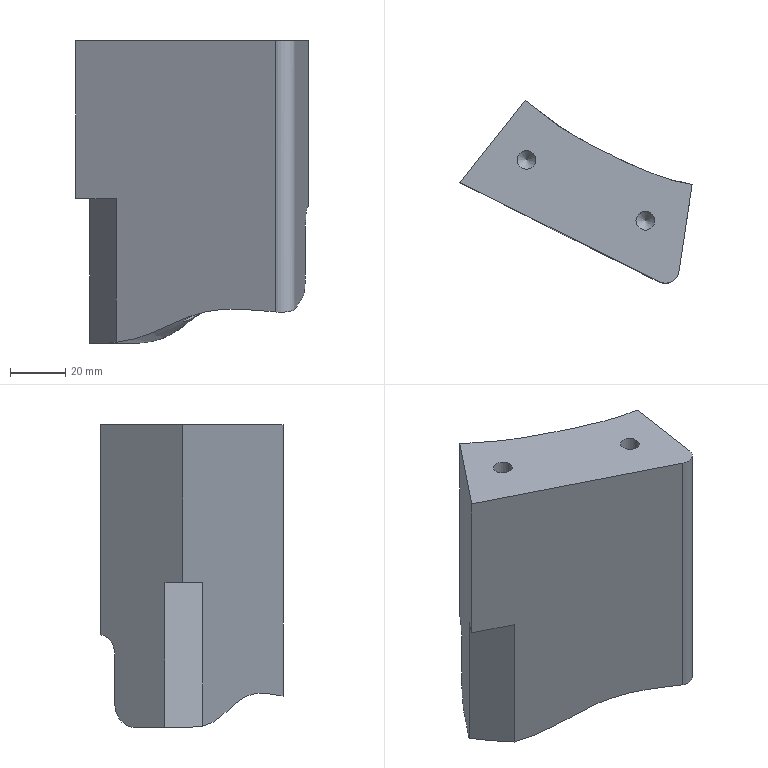Part | NX | features 8 2 | 1 solid | 31 faces | box 83.96 x 66.107 x 109.5 mm | volume 247036 mm3 | spline 11 | plane 9 | cylinder 7 | cone 3 | torus 1 | commonest cylinder face diameters 6.8 x2 8.5 x1 10 x1 14 x1 18 x1 240 x1